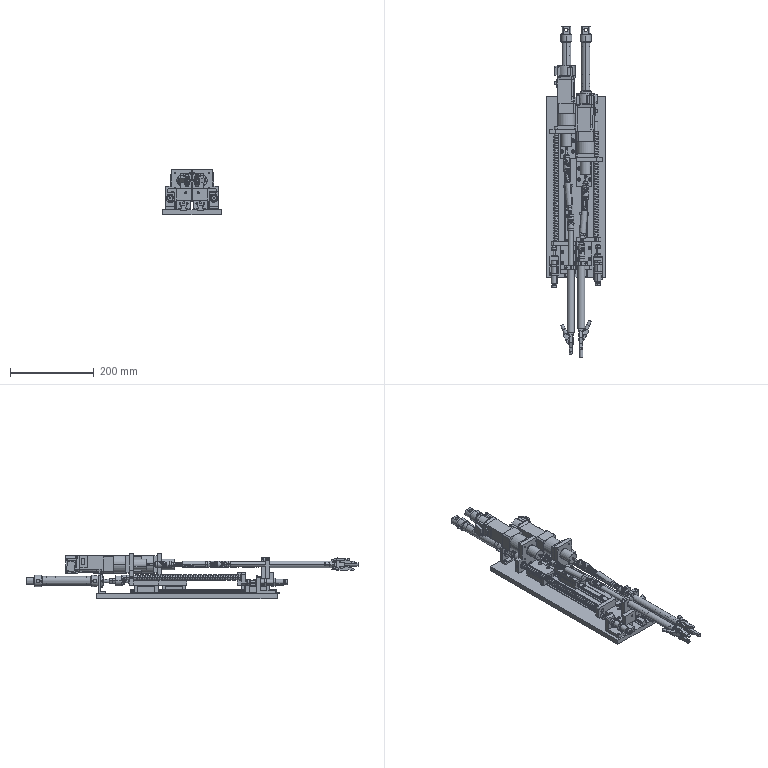Part | SolidWorks | 93 solids | 3628 faces | volume 1977709 mm3 | cylinder 1585 | plane 1443 | cone 472 | torus 64 | spline 32 | sphere 32 | commonest cylinder face diameters 8 x372 4 x112 3.5 x96 5 x86 4.5 x84 3.3 x60